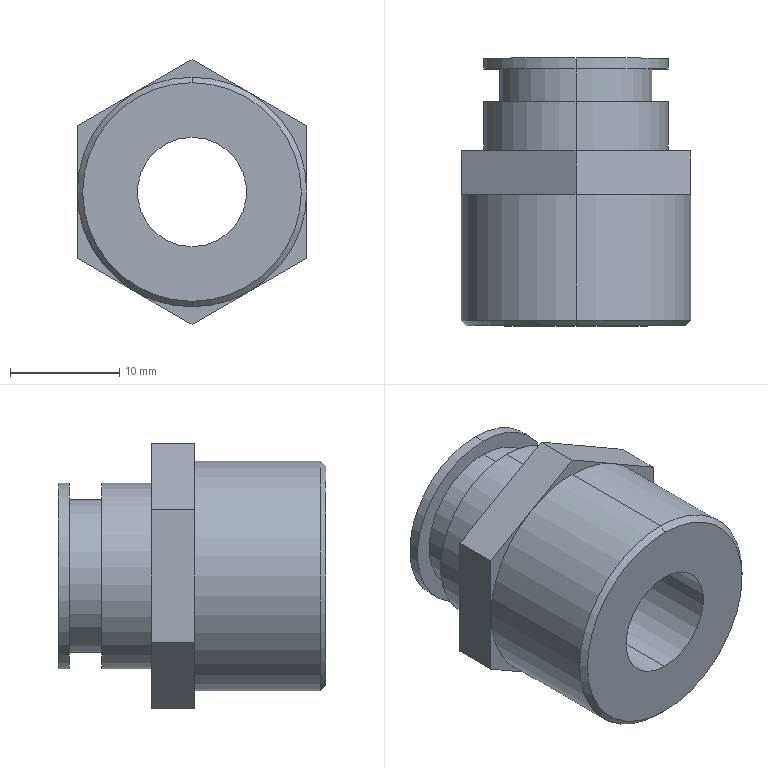Part | SolidWorks | features ICE 6, Chamfer 1, Extrusion 1 | 1 solid | 32 faces | box 21 x 24.5 x 24.249 mm | volume 5082 mm3 | plane 18 | cylinder 12 | cone 2 | commonest cylinder face diameters 17 x4 10 x2 12 x2 14 x2 21 x2
STEP:
#1=CARTESIAN_POINT('',(0.,13.5,-5.));
#2=VERTEX_POINT('',#1);
#3=CARTESIAN_POINT('',(0.,13.5,5.));
#4=VERTEX_POINT('',#3);
#5=CARTESIAN_POINT('',(0.,13.5,0.));
#6=DIRECTION('',(0.,1.,0.));
#7=DIRECTION('',(0.,0.,1.));
#8=AXIS2_PLACEMENT_3D('',#5,#6,#7);
#9=CIRCLE('',#8,5.);
#10=EDGE_CURVE('',#2,#4,#9,.T.);
#11=ORIENTED_EDGE('',*,*,#10,.T.);
#12=CARTESIAN_POINT('',(0.,0.,5.));
#13=VERTEX_POINT('',#12);
#14=CARTESIAN_POINT('',(0.,24.5,5.));
#15=DIRECTION('',(0.,-1.,0.));
#16=VECTOR('',#15,1000.);
#17=LINE('',#14,#16);
#18=EDGE_CURVE('',#4,#13,#17,.T.);
#19=ORIENTED_EDGE('',*,*,#18,.T.);
#20=CARTESIAN_POINT('',(0.,0.,-5.));
#21=VERTEX_POINT('',#20);
#22=CARTESIAN_POINT('',(0.,0.,0.));
#23=DIRECTION('',(0.,-1.,0.));
#24=DIRECTION('',(0.,0.,-1.));
#25=AXIS2_PLACEMENT_3D('',#22,#23,#24);
#26=CIRCLE('',#25,5.);
#27=EDGE_CURVE('',#13,#21,#26,.T.);
#28=ORIENTED_EDGE('',*,*,#27,.T.);
#29=CARTESIAN_POINT('',(0.,24.5,-5.));
#30=DIRECTION('',(0.,-1.,0.));
#31=VECTOR('',#30,1000.);
#32=LINE('',#29,#31);
#33=EDGE_CURVE('',#2,#21,#32,.T.);
#34=ORIENTED_EDGE('',*,*,#33,.F.);
#35=EDGE_LOOP('',(#11,#19,#28,#34));
#36=FACE_OUTER_BOUND('',#35,.T.);
#37=CARTESIAN_POINT('',(0.,24.5,0.));
#38=DIRECTION('',(0.,-1.,0.));
#39=DIRECTION('',(0.,0.,-1.));
#40=AXIS2_PLACEMENT_3D('',#37,#38,#39);
#41=CYLINDRICAL_SURFACE('',#40,5.);
#42=ADVANCED_FACE('',(#36),#41,.F.);
#43=CARTESIAN_POINT('',(0.,13.5,-6.));
#44=VERTEX_POINT('',#43);
#45=CARTESIAN_POINT('',(0.,13.5,6.));
#46=VERTEX_POINT('',#45);
#47=CARTESIAN_POINT('',(0.,13.5,0.));
#48=DIRECTION('',(0.,1.,0.));
#49=DIRECTION('',(0.,0.,1.));
#50=AXIS2_PLACEMENT_3D('',#47,#48,#49);
#51=CIRCLE('',#50,6.);
#52=EDGE_CURVE('',#44,#46,#51,.T.);
#53=ORIENTED_EDGE('',*,*,#52,.F.);
#54=CARTESIAN_POINT('',(0.,24.5,-6.));
#55=VERTEX_POINT('',#54);
#56=CARTESIAN_POINT('',(0.,13.5,-6.));
#57=DIRECTION('',(0.,1.,0.));
#58=VECTOR('',#57,1000.);
#59=LINE('',#56,#58);
#60=EDGE_CURVE('',#44,#55,#59,.T.);
#61=ORIENTED_EDGE('',*,*,#60,.T.);
#62=CARTESIAN_POINT('',(0.,24.5,6.));
#63=VERTEX_POINT('',#62);
#64=CARTESIAN_POINT('',(0.,24.5,0.));
#65=DIRECTION('',(0.,1.,0.));
#66=DIRECTION('',(0.,0.,1.));
#67=AXIS2_PLACEMENT_3D('',#64,#65,#66);
#68=CIRCLE('',#67,6.);
#69=EDGE_CURVE('',#55,#63,#68,.T.);
#70=ORIENTED_EDGE('',*,*,#69,.T.);
#71=CARTESIAN_POINT('',(0.,13.5,6.));
#72=DIRECTION('',(0.,1.,0.));
#73=VECTOR('',#72,1000.);
#74=LINE('',#71,#73);
#75=EDGE_CURVE('',#46,#63,#74,.T.);
#76=ORIENTED_EDGE('',*,*,#75,.F.);
#77=EDGE_LOOP('',(#53,#61,#70,#76));
#78=FACE_OUTER_BOUND('',#77,.T.);
#79=CARTESIAN_POINT('',(0.,13.5,0.));
#80=DIRECTION('',(0.,1.,0.));
#81=DIRECTION('',(0.,0.,1.));
#82=AXIS2_PLACEMENT_3D('',#79,#80,#81);
#83=CYLINDRICAL_SURFACE('',#82,6.);
#84=ADVANCED_FACE('',(#78),#83,.F.);
#85=CARTESIAN_POINT('',(0.,0.,-10.));
#86=VERTEX_POINT('',#85);
#87=CARTESIAN_POINT('',(0.,0.,10.));
#88=VERTEX_POINT('',#87);
#89=CARTESIAN_POINT('',(0.,0.,0.));
#90=DIRECTION('',(0.,-1.,0.));
#91=DIRECTION('',(0.,0.,1.));
#92=AXIS2_PLACEMENT_3D('',#89,#90,#91);
#93=CIRCLE('',#92,10.);
#94=EDGE_CURVE('',#86,#88,#93,.T.);
#95=ORIENTED_EDGE('',*,*,#94,.F.);
#96=CARTESIAN_POINT('',(0.,0.5,-10.5));
#97=VERTEX_POINT('',#96);
#98=CARTESIAN_POINT('',(0.,0.5,-10.5));
#99=DIRECTION('',(0.,0.7071,-0.7071));
#100=VECTOR('',#99,1000.);
#101=LINE('',#98,#100);
#102=EDGE_CURVE('',#86,#97,#101,.T.);
#103=ORIENTED_EDGE('',*,*,#102,.T.);
#104=CARTESIAN_POINT('',(0.,0.5,10.5));
#105=VERTEX_POINT('',#104);
#106=CARTESIAN_POINT('',(0.,0.5,0.));
#107=DIRECTION('',(0.,1.,0.));
#108=DIRECTION('',(0.,0.,1.));
#109=AXIS2_PLACEMENT_3D('',#106,#107,#108);
#110=CIRCLE('',#109,10.5);
#111=EDGE_CURVE('',#105,#97,#110,.T.);
#112=ORIENTED_EDGE('',*,*,#111,.F.);
#113=CARTESIAN_POINT('',(0.,0.5,10.5));
#114=DIRECTION('',(0.,0.7071,0.7071));
#115=VECTOR('',#114,1000.);
#116=LINE('',#113,#115);
#117=EDGE_CURVE('',#88,#105,#116,.T.);
#118=ORIENTED_EDGE('',*,*,#117,.F.);
#119=EDGE_LOOP('',(#95,#103,#112,#118));
#120=FACE_OUTER_BOUND('',#119,.T.);
#121=CARTESIAN_POINT('',(0.,0.5,0.));
#122=DIRECTION('',(0.,1.,0.));
#123=DIRECTION('',(0.,0.,1.));
#124=AXIS2_PLACEMENT_3D('',#121,#122,#123);
#125=CONICAL_SURFACE('',#124,10.5,0.7854);
#126=ADVANCED_FACE('',(#120),#125,.T.);
#127=CARTESIAN_POINT('',(0.,24.5,8.5));
#128=VERTEX_POINT('',#127);
#129=CARTESIAN_POINT('',(0.,24.5,-8.5));
#130=VERTEX_POINT('',#129);
#131=CARTESIAN_POINT('',(0.,24.5,0.));
#132=DIRECTION('',(0.,1.,0.));
#133=DIRECTION('',(0.,0.,1.));
#134=AXIS2_PLACEMENT_3D('',#131,#132,#133);
#135=CIRCLE('',#134,8.5);
#136=EDGE_CURVE('',#128,#130,#135,.T.);
#137=ORIENTED_EDGE('',*,*,#136,.F.);
#138=CARTESIAN_POINT('',(0.,23.5,8.5));
#139=VERTEX_POINT('',#138);
#140=CARTESIAN_POINT('',(0.,24.5,8.5));
#141=DIRECTION('',(0.,-1.,0.));
#142=VECTOR('',#141,1000.);
#143=LINE('',#140,#142);
#144=EDGE_CURVE('',#128,#139,#143,.T.);
#145=ORIENTED_EDGE('',*,*,#144,.T.);
#146=CARTESIAN_POINT('',(0.,23.5,-8.5));
#147=VERTEX_POINT('',#146);
#148=CARTESIAN_POINT('',(0.,23.5,0.));
#149=DIRECTION('',(0.,1.,0.));
#150=DIRECTION('',(0.,0.,1.));
#151=AXIS2_PLACEMENT_3D('',#148,#149,#150);
#152=CIRCLE('',#151,8.5);
#153=EDGE_CURVE('',#139,#147,#152,.T.);
#154=ORIENTED_EDGE('',*,*,#153,.T.);
#155=CARTESIAN_POINT('',(0.,24.5,-8.5));
#156=DIRECTION('',(0.,-1.,0.));
#157=VECTOR('',#156,1000.);
#158=LINE('',#155,#157);
#159=EDGE_CURVE('',#130,#147,#158,.T.);
#160=ORIENTED_EDGE('',*,*,#159,.F.);
#161=EDGE_LOOP('',(#137,#145,#154,#160));
#162=FACE_OUTER_BOUND('',#161,.T.);
#163=CARTESIAN_POINT('',(0.,24.5,0.));
#164=DIRECTION('',(0.,-1.,0.));
#165=DIRECTION('',(0.,0.,-1.));
#166=AXIS2_PLACEMENT_3D('',#163,#164,#165);
#167=CYLINDRICAL_SURFACE('',#166,8.5);
#168=ADVANCED_FACE('',(#162),#167,.T.);
#169=CARTESIAN_POINT('',(0.,23.5,7.));
#170=VERTEX_POINT('',#169);
#171=CARTESIAN_POINT('',(0.,23.5,-7.));
#172=VERTEX_POINT('',#171);
#173=CARTESIAN_POINT('',(0.,23.5,0.));
#174=DIRECTION('',(0.,1.,0.));
#175=DIRECTION('',(0.,0.,1.));
#176=AXIS2_PLACEMENT_3D('',#173,#174,#175);
#177=CIRCLE('',#176,7.);
#178=EDGE_CURVE('',#170,#172,#177,.T.);
#179=ORIENTED_EDGE('',*,*,#178,.F.);
#180=CARTESIAN_POINT('',(0.,20.5,7.));
#181=VERTEX_POINT('',#180);
#182=CARTESIAN_POINT('',(0.,23.5,7.));
#183=DIRECTION('',(0.,-1.,0.));
#184=VECTOR('',#183,1000.);
#185=LINE('',#182,#184);
#186=EDGE_CURVE('',#170,#181,#185,.T.);
#187=ORIENTED_EDGE('',*,*,#186,.T.);
#188=CARTESIAN_POINT('',(0.,20.5,-7.));
#189=VERTEX_POINT('',#188);
#190=CARTESIAN_POINT('',(0.,20.5,0.));
#191=DIRECTION('',(0.,1.,0.));
#192=DIRECTION('',(0.,0.,1.));
#193=AXIS2_PLACEMENT_3D('',#190,#191,#192);
#194=CIRCLE('',#193,7.);
#195=EDGE_CURVE('',#181,#189,#194,.T.);
#196=ORIENTED_EDGE('',*,*,#195,.T.);
#197=CARTESIAN_POINT('',(0.,23.5,-7.));
#198=DIRECTION('',(0.,-1.,0.));
#199=VECTOR('',#198,1000.);
#200=LINE('',#197,#199);
#201=EDGE_CURVE('',#172,#189,#200,.T.);
#202=ORIENTED_EDGE('',*,*,#201,.F.);
#203=EDGE_LOOP('',(#179,#187,#196,#202));
#204=FACE_OUTER_BOUND('',#203,.T.);
#205=CARTESIAN_POINT('',(0.,23.5,0.));
#206=DIRECTION('',(0.,-1.,0.));
#207=DIRECTION('',(0.,0.,-1.));
#208=AXIS2_PLACEMENT_3D('',#205,#206,#207);
#209=CYLINDRICAL_SURFACE('',#208,7.);
#210=ADVANCED_FACE('',(#204),#209,.T.);
#211=CARTESIAN_POINT('',(0.,20.5,8.5));
#212=VERTEX_POINT('',#211);
#213=CARTESIAN_POINT('',(0.,20.5,-8.5));
#214=VERTEX_POINT('',#213);
#215=CARTESIAN_POINT('',(0.,20.5,0.));
#216=DIRECTION('',(0.,1.,0.));
#217=DIRECTION('',(0.,0.,1.));
#218=AXIS2_PLACEMENT_3D('',#215,#216,#217);
#219=CIRCLE('',#218,8.5);
#220=EDGE_CURVE('',#212,#214,#219,.T.);
#221=ORIENTED_EDGE('',*,*,#220,.F.);
#222=CARTESIAN_POINT('',(0.,16.,8.5));
#223=VERTEX_POINT('',#222);
#224=CARTESIAN_POINT('',(0.,20.5,8.5));
#225=DIRECTION('',(0.,-1.,0.));
#226=VECTOR('',#225,1000.);
#227=LINE('',#224,#226);
#228=EDGE_CURVE('',#212,#223,#227,.T.);
#229=ORIENTED_EDGE('',*,*,#228,.T.);
#230=CARTESIAN_POINT('',(0.,16.,-8.5));
#231=VERTEX_POINT('',#230);
#232=CARTESIAN_POINT('',(0.,16.,0.));
#233=DIRECTION('',(0.,1.,0.));
#234=DIRECTION('',(0.,0.,1.));
#235=AXIS2_PLACEMENT_3D('',#232,#233,#234);
#236=CIRCLE('',#235,8.5);
#237=EDGE_CURVE('',#223,#231,#236,.T.);
#238=ORIENTED_EDGE('',*,*,#237,.T.);
#239=CARTESIAN_POINT('',(0.,20.5,-8.5));
#240=DIRECTION('',(0.,-1.,0.));
#241=VECTOR('',#240,1000.);
#242=LINE('',#239,#241);
#243=EDGE_CURVE('',#214,#231,#242,.T.);
#244=ORIENTED_EDGE('',*,*,#243,.F.);
#245=EDGE_LOOP('',(#221,#229,#238,#244));
#246=FACE_OUTER_BOUND('',#245,.T.);
#247=CARTESIAN_POINT('',(0.,20.5,0.));
#248=DIRECTION('',(0.,-1.,0.));
#249=DIRECTION('',(0.,0.,-1.));
#250=AXIS2_PLACEMENT_3D('',#247,#248,#249);
#251=CYLINDRICAL_SURFACE('',#250,8.5);
#252=ADVANCED_FACE('',(#246),#251,.T.);
#253=CARTESIAN_POINT('',(0.,12.,10.5));
#254=VERTEX_POINT('',#253);
#255=CARTESIAN_POINT('',(5.25,12.,9.093));
#256=VERTEX_POINT('',#255);
#257=CARTESIAN_POINT('',(0.,12.,0.));
#258=DIRECTION('',(0.,1.,0.));
#259=DIRECTION('',(0.,0.,1.));
#260=AXIS2_PLACEMENT_3D('',#257,#258,#259);
#261=CIRCLE('',#260,10.5);
#262=EDGE_CURVE('',#254,#256,#261,.T.);
#263=ORIENTED_EDGE('',*,*,#262,.F.);
#264=CARTESIAN_POINT('',(0.,12.,10.5));
#265=DIRECTION('',(0.,-1.,0.));
#266=VECTOR('',#265,1000.);
#267=LINE('',#264,#266);
#268=EDGE_CURVE('',#254,#105,#267,.T.);
#269=ORIENTED_EDGE('',*,*,#268,.T.);
#270=ORIENTED_EDGE('',*,*,#111,.T.);
#271=CARTESIAN_POINT('',(0.,12.,-10.5));
#272=VERTEX_POINT('',#271);
#273=CARTESIAN_POINT('',(0.,12.,-10.5));
#274=DIRECTION('',(0.,-1.,0.));
#275=VECTOR('',#274,1000.);
#276=LINE('',#273,#275);
#277=EDGE_CURVE('',#272,#97,#276,.T.);
#278=ORIENTED_EDGE('',*,*,#277,.F.);
#279=CARTESIAN_POINT('',(5.25,12.,-9.093));
#280=VERTEX_POINT('',#279);
#281=CARTESIAN_POINT('',(0.,12.,0.));
#282=DIRECTION('',(0.,1.,0.));
#283=DIRECTION('',(0.,0.,1.));
#284=AXIS2_PLACEMENT_3D('',#281,#282,#283);
#285=CIRCLE('',#284,10.5);
#286=EDGE_CURVE('',#280,#272,#285,.T.);
#287=ORIENTED_EDGE('',*,*,#286,.F.);
#288=CARTESIAN_POINT('',(10.5,12.,0.));
#289=VERTEX_POINT('',#288);
#290=CARTESIAN_POINT('',(0.,12.,0.));
#291=DIRECTION('',(0.,1.,0.));
#292=DIRECTION('',(0.,0.,1.));
#293=AXIS2_PLACEMENT_3D('',#290,#291,#292);
#294=CIRCLE('',#293,10.5);
#295=EDGE_CURVE('',#289,#280,#294,.T.);
#296=ORIENTED_EDGE('',*,*,#295,.F.);
#297=CARTESIAN_POINT('',(0.,12.,0.));
#298=DIRECTION('',(0.,1.,0.));
#299=DIRECTION('',(0.,0.,1.));
#300=AXIS2_PLACEMENT_3D('',#297,#298,#299);
#301=CIRCLE('',#300,10.5);
#302=EDGE_CURVE('',#256,#289,#301,.T.);
#303=ORIENTED_EDGE('',*,*,#302,.F.);
#304=EDGE_LOOP('',(#263,#269,#270,#278,#287,#296,#303));
#305=FACE_OUTER_BOUND('',#304,.T.);
#306=CARTESIAN_POINT('',(0.,12.,0.));
#307=DIRECTION('',(0.,-1.,0.));
#308=DIRECTION('',(0.,0.,-1.));
#309=AXIS2_PLACEMENT_3D('',#306,#307,#308);
#310=CYLINDRICAL_SURFACE('',#309,10.5);
#311=ADVANCED_FACE('',(#305),#310,.T.);
#312=ORIENTED_EDGE('',*,*,#268,.F.);
#313=CARTESIAN_POINT('',(-5.25,12.,9.093));
#314=VERTEX_POINT('',#313);
#315=CARTESIAN_POINT('',(0.,12.,0.));
#316=DIRECTION('',(0.,1.,0.));
#317=DIRECTION('',(0.,0.,1.));
#318=AXIS2_PLACEMENT_3D('',#315,#316,#317);
#319=CIRCLE('',#318,10.5);
#320=EDGE_CURVE('',#314,#254,#319,.T.);
#321=ORIENTED_EDGE('',*,*,#320,.F.);
#322=CARTESIAN_POINT('',(-10.5,12.,0.));
#323=VERTEX_POINT('',#322);
#324=CARTESIAN_POINT('',(0.,12.,0.));
#325=DIRECTION('',(0.,1.,0.));
#326=DIRECTION('',(0.,0.,1.));
#327=AXIS2_PLACEMENT_3D('',#324,#325,#326);
#328=CIRCLE('',#327,10.5);
#329=EDGE_CURVE('',#323,#314,#328,.T.);
#330=ORIENTED_EDGE('',*,*,#329,.F.);
#331=CARTESIAN_POINT('',(-5.25,12.,-9.093));
#332=VERTEX_POINT('',#331);
#333=CARTESIAN_POINT('',(0.,12.,0.));
#334=DIRECTION('',(0.,1.,0.));
#335=DIRECTION('',(0.,0.,1.));
#336=AXIS2_PLACEMENT_3D('',#333,#334,#335);
#337=CIRCLE('',#336,10.5);
#338=EDGE_CURVE('',#332,#323,#337,.T.);
#339=ORIENTED_EDGE('',*,*,#338,.F.);
#340=CARTESIAN_POINT('',(0.,12.,0.));
#341=DIRECTION('',(0.,1.,0.));
#342=DIRECTION('',(0.,0.,1.));
#343=AXIS2_PLACEMENT_3D('',#340,#341,#342);
#344=CIRCLE('',#343,10.5);
#345=EDGE_CURVE('',#272,#332,#344,.T.);
#346=ORIENTED_EDGE('',*,*,#345,.F.);
#347=ORIENTED_EDGE('',*,*,#277,.T.);
#348=CARTESIAN_POINT('',(0.,0.5,0.));
#349=DIRECTION('',(0.,1.,0.));
#350=DIRECTION('',(0.,0.,1.));
#351=AXIS2_PLACEMENT_3D('',#348,#349,#350);
#352=CIRCLE('',#351,10.5);
#353=EDGE_CURVE('',#97,#105,#352,.T.);
#354=ORIENTED_EDGE('',*,*,#353,.T.);
#355=EDGE_LOOP('',(#312,#321,#330,#339,#346,#347,#354));
#356=FACE_OUTER_BOUND('',#355,.T.);
#357=CARTESIAN_POINT('',(0.,12.,0.));
#358=DIRECTION('',(0.,-1.,0.));
#359=DIRECTION('',(0.,0.,-1.));
#360=AXIS2_PLACEMENT_3D('',#357,#358,#359);
#361=CYLINDRICAL_SURFACE('',#360,10.5);
#362=ADVANCED_FACE('',(#356),#361,.T.);
#363=CARTESIAN_POINT('',(0.,0.,0.));
#364=DIRECTION('',(0.,-1.,0.));
#365=DIRECTION('',(0.,0.,-1.));
#366=AXIS2_PLACEMENT_3D('',#363,#364,#365);
#367=CIRCLE('',#366,5.);
#368=EDGE_CURVE('',#21,#13,#367,.T.);
#369=ORIENTED_EDGE('',*,*,#368,.F.);
#370=ORIENTED_EDGE('',*,*,#27,.F.);
#371=EDGE_LOOP('',(#369,#370));
#372=FACE_BOUND('',#371,.T.);
#373=CARTESIAN_POINT('',(0.,0.,0.));
#374=DIRECTION('',(0.,-1.,0.));
#375=DIRECTION('',(0.,0.,1.));
#376=AXIS2_PLACEMENT_3D('',#373,#374,#375);
#377=CIRCLE('',#376,10.);
#378=EDGE_CURVE('',#88,#86,#377,.T.);
#379=ORIENTED_EDGE('',*,*,#378,.T.);
#380=ORIENTED_EDGE('',*,*,#94,.T.);
#381=EDGE_LOOP('',(#379,#380));
#382=FACE_OUTER_BOUND('',#381,.T.);
#383=CARTESIAN_POINT('',(0.,0.,0.));
#384=DIRECTION('',(0.,1.,0.));
#385=DIRECTION('',(0.,0.,1.));
#386=AXIS2_PLACEMENT_3D('',#383,#384,#385);
#387=PLANE('',#386);
#388=ADVANCED_FACE('',(#372,#382),#387,.F.);
#389=CARTESIAN_POINT('',(10.5,12.,6.062));
#390=VERTEX_POINT('',#389);
#391=CARTESIAN_POINT('',(0.,12.,12.124));
#392=DIRECTION('',(0.866,0.,-0.5));
#393=VECTOR('',#392,1000.);
#394=LINE('',#391,#393);
#395=EDGE_CURVE('',#256,#390,#394,.T.);
#396=ORIENTED_EDGE('',*,*,#395,.F.);
#397=ORIENTED_EDGE('',*,*,#302,.T.);
#398=CARTESIAN_POINT('',(10.5,12.,6.062));
#399=DIRECTION('',(0.,0.,-1.));
#400=VECTOR('',#399,1000.);
#401=LINE('',#398,#400);
#402=EDGE_CURVE('',#390,#289,#401,.T.);
#403=ORIENTED_EDGE('',*,*,#402,.F.);
#404=EDGE_LOOP('',(#396,#397,#403));
#405=FACE_OUTER_BOUND('',#404,.T.);
#406=CARTESIAN_POINT('',(0.,12.,0.));
#407=DIRECTION('',(0.,1.,0.));
#408=DIRECTION('',(0.,0.,1.));
#409=AXIS2_PLACEMENT_3D('',#406,#407,#408);
#410=PLANE('',#409);
#411=ADVANCED_FACE('',(#405),#410,.F.);
#412=CARTESIAN_POINT('',(10.5,12.,-6.062));
#413=VERTEX_POINT('',#412);
#414=CARTESIAN_POINT('',(10.5,12.,6.062));
#415=DIRECTION('',(0.,0.,-1.));
#416=VECTOR('',#415,1000.);
#417=LINE('',#414,#416);
#418=EDGE_CURVE('',#289,#413,#417,.T.);
#419=ORIENTED_EDGE('',*,*,#418,.F.);
#420=ORIENTED_EDGE('',*,*,#295,.T.);
#421=CARTESIAN_POINT('',(10.5,12.,-6.062));
#422=DIRECTION('',(-0.866,0.,-0.5));
#423=VECTOR('',#422,1000.);
#424=LINE('',#421,#423);
#425=EDGE_CURVE('',#413,#280,#424,.T.);
#426=ORIENTED_EDGE('',*,*,#425,.F.);
#427=EDGE_LOOP('',(#419,#420,#426));
#428=FACE_OUTER_BOUND('',#427,.T.);
#429=CARTESIAN_POINT('',(0.,12.,0.));
#430=DIRECTION('',(0.,1.,0.));
#431=DIRECTION('',(0.,0.,1.));
#432=AXIS2_PLACEMENT_3D('',#429,#430,#431);
#433=PLANE('',#432);
#434=ADVANCED_FACE('',(#428),#433,.F.);
#435=CARTESIAN_POINT('',(0.,12.,-12.124));
#436=VERTEX_POINT('',#435);
#437=CARTESIAN_POINT('',(10.5,12.,-6.062));
#438=DIRECTION('',(-0.866,0.,-0.5));
#439=VECTOR('',#438,1000.);
#440=LINE('',#437,#439);
#441=EDGE_CURVE('',#280,#436,#440,.T.);
#442=ORIENTED_EDGE('',*,*,#441,.F.);
#443=ORIENTED_EDGE('',*,*,#286,.T.);
#444=ORIENTED_EDGE('',*,*,#345,.T.);
#445=CARTESIAN_POINT('',(0.,12.,-12.124));
#446=DIRECTION('',(-0.866,0.,0.5));
#447=VECTOR('',#446,1000.);
#448=LINE('',#445,#447);
#449=EDGE_CURVE('',#436,#332,#448,.T.);
#450=ORIENTED_EDGE('',*,*,#449,.F.);
#451=EDGE_LOOP('',(#442,#443,#444,#450));
#452=FACE_OUTER_BOUND('',#451,.T.);
#453=CARTESIAN_POINT('',(0.,12.,0.));
#454=DIRECTION('',(0.,1.,0.));
#455=DIRECTION('',(0.,0.,1.));
#456=AXIS2_PLACEMENT_3D('',#453,#454,#455);
#457=PLANE('',#456);
#458=ADVANCED_FACE('',(#452),#457,.F.);
#459=CARTESIAN_POINT('',(-10.5,12.,-6.062));
#460=VERTEX_POINT('',#459);
#461=CARTESIAN_POINT('',(0.,12.,-12.124));
#462=DIRECTION('',(-0.866,0.,0.5));
#463=VECTOR('',#462,1000.);
#464=LINE('',#461,#463);
#465=EDGE_CURVE('',#332,#460,#464,.T.);
#466=ORIENTED_EDGE('',*,*,#465,.F.);
#467=ORIENTED_EDGE('',*,*,#338,.T.);
#468=CARTESIAN_POINT('',(-10.5,12.,-6.062));
#469=DIRECTION('',(0.,0.,1.));
#470=VECTOR('',#469,1000.);
#471=LINE('',#468,#470);
#472=EDGE_CURVE('',#460,#323,#471,.T.);
#473=ORIENTED_EDGE('',*,*,#472,.F.);
#474=EDGE_LOOP('',(#466,#467,#473));
#475=FACE_OUTER_BOUND('',#474,.T.);
#476=CARTESIAN_POINT('',(0.,12.,0.));
#477=DIRECTION('',(0.,1.,0.));
#478=DIRECTION('',(0.,0.,1.));
#479=AXIS2_PLACEMENT_3D('',#476,#477,#478);
#480=PLANE('',#479);
#481=ADVANCED_FACE('',(#475),#480,.F.);
#482=CARTESIAN_POINT('',(-10.5,12.,6.062));
#483=VERTEX_POINT('',#482);
#484=CARTESIAN_POINT('',(-10.5,12.,-6.062));
#485=DIRECTION('',(0.,0.,1.));
#486=VECTOR('',#485,1000.);
#487=LINE('',#484,#486);
#488=EDGE_CURVE('',#323,#483,#487,.T.);
#489=ORIENTED_EDGE('',*,*,#488,.F.);
#490=ORIENTED_EDGE('',*,*,#329,.T.);
#491=CARTESIAN_POINT('',(-10.5,12.,6.062));
#492=DIRECTION('',(0.866,0.,0.5));
#493=VECTOR('',#492,1000.);
#494=LINE('',#491,#493);
#495=EDGE_CURVE('',#483,#314,#494,.T.);
#496=ORIENTED_EDGE('',*,*,#495,.F.);
#497=EDGE_LOOP('',(#489,#490,#496));
#498=FACE_OUTER_BOUND('',#497,.T.);
#499=CARTESIAN_POINT('',(0.,12.,0.));
#500=DIRECTION('',(0.,1.,0.));
#501=DIRECTION('',(0.,0.,1.));
#502=AXIS2_PLACEMENT_3D('',#499,#500,#501);
#503=PLANE('',#502);
#504=ADVANCED_FACE('',(#498),#503,.F.);
#505=CARTESIAN_POINT('',(0.,12.,12.124));
#506=VERTEX_POINT('',#505);
#507=CARTESIAN_POINT('',(-10.5,12.,6.062));
#508=DIRECTION('',(0.866,0.,0.5));
#509=VECTOR('',#508,1000.);
#510=LINE('',#507,#509);
#511=EDGE_CURVE('',#314,#506,#510,.T.);
#512=ORIENTED_EDGE('',*,*,#511,.F.);
#513=ORIENTED_EDGE('',*,*,#320,.T.);
#514=ORIENTED_EDGE('',*,*,#262,.T.);
#515=CARTESIAN_POINT('',(0.,12.,12.124));
#516=DIRECTION('',(0.866,0.,-0.5));
#517=VECTOR('',#516,1000.);
#518=LINE('',#515,#517);
#519=EDGE_CURVE('',#506,#256,#518,.T.);
#520=ORIENTED_EDGE('',*,*,#519,.F.);
#521=EDGE_LOOP('',(#512,#513,#514,#520));
#522=FACE_OUTER_BOUND('',#521,.T.);
#523=CARTESIAN_POINT('',(0.,12.,0.));
#524=DIRECTION('',(0.,1.,0.));
#525=DIRECTION('',(0.,0.,1.));
#526=AXIS2_PLACEMENT_3D('',#523,#524,#525);
#527=PLANE('',#526);
#528=ADVANCED_FACE('',(#522),#527,.F.);
#529=ORIENTED_EDGE('',*,*,#519,.T.);
#530=ORIENTED_EDGE('',*,*,#395,.T.);
#531=CARTESIAN_POINT('',(10.5,16.,6.062));
#532=VERTEX_POINT('',#531);
#533=CARTESIAN_POINT('',(10.5,16.,6.062));
#534=DIRECTION('',(0.,-1.,0.));
#535=VECTOR('',#534,1000.);
#536=LINE('',#533,#535);
#537=EDGE_CURVE('',#532,#390,#536,.T.);
#538=ORIENTED_EDGE('',*,*,#537,.F.);
#539=CARTESIAN_POINT('',(0.,16.,12.124));
#540=VERTEX_POINT('',#539);
#541=CARTESIAN_POINT('',(0.,16.,12.124));
#542=DIRECTION('',(0.866,0.,-0.5));
#543=VECTOR('',#542,1000.);
#544=LINE('',#541,#543);
#545=EDGE_CURVE('',#540,#532,#544,.T.);
#546=ORIENTED_EDGE('',*,*,#545,.F.);
#547=CARTESIAN_POINT('',(0.,16.,12.124));
#548=DIRECTION('',(0.,-1.,0.));
#549=VECTOR('',#548,1000.);
#550=LINE('',#547,#549);
#551=EDGE_CURVE('',#540,#506,#550,.T.);
#552=ORIENTED_EDGE('',*,*,#551,.T.);
#553=EDGE_LOOP('',(#529,#530,#538,#546,#552));
#554=FACE_OUTER_BOUND('',#553,.T.);
#555=CARTESIAN_POINT('',(0.,16.,12.124));
#556=DIRECTION('',(-0.5,0.,-0.866));
#557=DIRECTION('',(-0.866,0.,0.5));
#558=AXIS2_PLACEMENT_3D('',#555,#556,#557);
#559=PLANE('',#558);
#560=ADVANCED_FACE('',(#554),#559,.F.);
#561=ORIENTED_EDGE('',*,*,#402,.T.);
#562=ORIENTED_EDGE('',*,*,#418,.T.);
#563=CARTESIAN_POINT('',(10.5,16.,-6.062));
#564=VERTEX_POINT('',#563);
#565=CARTESIAN_POINT('',(10.5,16.,-6.062));
#566=DIRECTION('',(0.,-1.,0.));
#567=VECTOR('',#566,1000.);
#568=LINE('',#565,#567);
#569=EDGE_CURVE('',#564,#413,#568,.T.);
#570=ORIENTED_EDGE('',*,*,#569,.F.);
#571=CARTESIAN_POINT('',(10.5,16.,6.062));
#572=DIRECTION('',(0.,0.,-1.));
#573=VECTOR('',#572,1000.);
#574=LINE('',#571,#573);
#575=EDGE_CURVE('',#532,#564,#574,.T.);
#576=ORIENTED_EDGE('',*,*,#575,.F.);
#577=ORIENTED_EDGE('',*,*,#537,.T.);
#578=EDGE_LOOP('',(#561,#562,#570,#576,#577));
#579=FACE_OUTER_BOUND('',#578,.T.);
#580=CARTESIAN_POINT('',(10.5,16.,6.062));
#581=DIRECTION('',(-1.,0.,0.));
#582=DIRECTION('',(0.,0.,1.));
#583=AXIS2_PLACEMENT_3D('',#580,#581,#582);
#584=PLANE('',#583);
#585=ADVANCED_FACE('',(#579),#584,.F.);
#586=ORIENTED_EDGE('',*,*,#425,.T.);
#587=ORIENTED_EDGE('',*,*,#441,.T.);
#588=CARTESIAN_POINT('',(0.,16.,-12.124));
#589=VERTEX_POINT('',#588);
#590=CARTESIAN_POINT('',(0.,16.,-12.124));
#591=DIRECTION('',(0.,-1.,0.));
#592=VECTOR('',#591,1000.);
#593=LINE('',#590,#592);
#594=EDGE_CURVE('',#589,#436,#593,.T.);
#595=ORIENTED_EDGE('',*,*,#594,.F.);
#596=CARTESIAN_POINT('',(10.5,16.,-6.062));
#597=DIRECTION('',(-0.866,0.,-0.5));
#598=VECTOR('',#597,1000.);
#599=LINE('',#596,#598);
#600=EDGE_CURVE('',#564,#589,#599,.T.);
#601=ORIENTED_EDGE('',*,*,#600,.F.);
#602=ORIENTED_EDGE('',*,*,#569,.T.);
#603=EDGE_LOOP('',(#586,#587,#595,#601,#602));
#604=FACE_OUTER_BOUND('',#603,.T.);
#605=CARTESIAN_POINT('',(10.5,16.,-6.062));
#606=DIRECTION('',(-0.5,0.,0.866));
#607=DIRECTION('',(0.866,0.,0.5));
#608=AXIS2_PLACEMENT_3D('',#605,#606,#607);
#609=PLANE('',#608);
#610=ADVANCED_FACE('',(#604),#609,.F.);
#611=ORIENTED_EDGE('',*,*,#449,.T.);
#612=ORIENTED_EDGE('',*,*,#465,.T.);
#613=CARTESIAN_POINT('',(-10.5,16.,-6.062));
#614=VERTEX_POINT('',#613);
#615=CARTESIAN_POINT('',(-10.5,16.,-6.062));
#616=DIRECTION('',(0.,-1.,0.));
#617=VECTOR('',#616,1000.);
#618=LINE('',#615,#617);
#619=EDGE_CURVE('',#614,#460,#618,.T.);
#620=ORIENTED_EDGE('',*,*,#619,.F.);
#621=CARTESIAN_POINT('',(0.,16.,-12.124));
#622=DIRECTION('',(-0.866,0.,0.5));
#623=VECTOR('',#622,1000.);
#624=LINE('',#621,#623);
#625=EDGE_CURVE('',#589,#614,#624,.T.);
#626=ORIENTED_EDGE('',*,*,#625,.F.);
#627=ORIENTED_EDGE('',*,*,#594,.T.);
#628=EDGE_LOOP('',(#611,#612,#620,#626,#627));
#629=FACE_OUTER_BOUND('',#628,.T.);
#630=CARTESIAN_POINT('',(0.,16.,-12.124));
#631=DIRECTION('',(0.5,0.,0.866));
#632=DIRECTION('',(0.866,0.,-0.5));
#633=AXIS2_PLACEMENT_3D('',#630,#631,#632);
#634=PLANE('',#633);
#635=ADVANCED_FACE('',(#629),#634,.F.);
#636=ORIENTED_EDGE('',*,*,#472,.T.);
#637=ORIENTED_EDGE('',*,*,#488,.T.);
#638=CARTESIAN_POINT('',(-10.5,16.,6.062));
#639=VERTEX_POINT('',#638);
#640=CARTESIAN_POINT('',(-10.5,16.,6.062));
#641=DIRECTION('',(0.,-1.,0.));
#642=VECTOR('',#641,1000.);
#643=LINE('',#640,#642);
#644=EDGE_CURVE('',#639,#483,#643,.T.);
#645=ORIENTED_EDGE('',*,*,#644,.F.);
#646=CARTESIAN_POINT('',(-10.5,16.,-6.062));
#647=DIRECTION('',(0.,0.,1.));
#648=VECTOR('',#647,1000.);
#649=LINE('',#646,#648);
#650=EDGE_CURVE('',#614,#639,#649,.T.);
#651=ORIENTED_EDGE('',*,*,#650,.F.);
#652=ORIENTED_EDGE('',*,*,#619,.T.);
#653=EDGE_LOOP('',(#636,#637,#645,#651,#652));
#654=FACE_OUTER_BOUND('',#653,.T.);
#655=CARTESIAN_POINT('',(-10.5,16.,-6.062));
#656=DIRECTION('',(1.,0.,0.));
#657=DIRECTION('',(0.,0.,-1.));
#658=AXIS2_PLACEMENT_3D('',#655,#656,#657);
#659=PLANE('',#658);
#660=ADVANCED_FACE('',(#654),#659,.F.);
#661=ORIENTED_EDGE('',*,*,#495,.T.);
#662=ORIENTED_EDGE('',*,*,#511,.T.);
#663=ORIENTED_EDGE('',*,*,#551,.F.);
#664=CARTESIAN_POINT('',(-10.5,16.,6.062));
#665=DIRECTION('',(0.866,0.,0.5));
#666=VECTOR('',#665,1000.);
#667=LINE('',#664,#666);
#668=EDGE_CURVE('',#639,#540,#667,.T.);
#669=ORIENTED_EDGE('',*,*,#668,.F.);
#670=ORIENTED_EDGE('',*,*,#644,.T.);
#671=EDGE_LOOP('',(#661,#662,#663,#669,#670));
#672=FACE_OUTER_BOUND('',#671,.T.);
#673=CARTESIAN_POINT('',(-10.5,16.,6.062));
#674=DIRECTION('',(0.5,0.,-0.866));
#675=DIRECTION('',(-0.866,0.,-0.5));
#676=AXIS2_PLACEMENT_3D('',#673,#674,#675);
#677=PLANE('',#676);
#678=ADVANCED_FACE('',(#672),#677,.F.);
#679=CARTESIAN_POINT('',(0.,16.,0.));
#680=DIRECTION('',(0.,1.,0.));
#681=DIRECTION('',(0.,0.,1.));
#682=AXIS2_PLACEMENT_3D('',#679,#680,#681);
#683=CIRCLE('',#682,8.5);
#684=EDGE_CURVE('',#231,#223,#683,.T.);
#685=ORIENTED_EDGE('',*,*,#684,.F.);
#686=ORIENTED_EDGE('',*,*,#237,.F.);
#687=EDGE_LOOP('',(#685,#686));
#688=FACE_BOUND('',#687,.T.);
#689=ORIENTED_EDGE('',*,*,#545,.T.);
#690=ORIENTED_EDGE('',*,*,#575,.T.);
#691=ORIENTED_EDGE('',*,*,#600,.T.);
#692=ORIENTED_EDGE('',*,*,#625,.T.);
#693=ORIENTED_EDGE('',*,*,#650,.T.);
#694=ORIENTED_EDGE('',*,*,#668,.T.);
#695=EDGE_LOOP('',(#689,#690,#691,#692,#693,#694));
#696=FACE_OUTER_BOUND('',#695,.T.);
#697=CARTESIAN_POINT('',(0.,16.,0.));
#698=DIRECTION('',(0.,1.,0.));
#699=DIRECTION('',(0.,0.,1.));
#700=AXIS2_PLACEMENT_3D('',#697,#698,#699);
#701=PLANE('',#700);
#702=ADVANCED_FACE('',(#688,#696),#701,.T.);
#703=ORIENTED_EDGE('',*,*,#228,.F.);
#704=CARTESIAN_POINT('',(0.,20.5,0.));
#705=DIRECTION('',(0.,1.,0.));
#706=DIRECTION('',(0.,0.,1.));
#707=AXIS2_PLACEMENT_3D('',#704,#705,#706);
#708=CIRCLE('',#707,8.5);
#709=EDGE_CURVE('',#214,#212,#708,.T.);
#710=ORIENTED_EDGE('',*,*,#709,.F.);
#711=ORIENTED_EDGE('',*,*,#243,.T.);
#712=ORIENTED_EDGE('',*,*,#684,.T.);
#713=EDGE_LOOP('',(#703,#710,#711,#712));
#714=FACE_OUTER_BOUND('',#713,.T.);
#715=CARTESIAN_POINT('',(0.,20.5,0.));
#716=DIRECTION('',(0.,-1.,0.));
#717=DIRECTION('',(0.,0.,-1.));
#718=AXIS2_PLACEMENT_3D('',#715,#716,#717);
#719=CYLINDRICAL_SURFACE('',#718,8.5);
#720=ADVANCED_FACE('',(#714),#719,.T.);
#721=CARTESIAN_POINT('',(0.,20.5,0.));
#722=DIRECTION('',(0.,1.,0.));
#723=DIRECTION('',(0.,0.,1.));
#724=AXIS2_PLACEMENT_3D('',#721,#722,#723);
#725=CIRCLE('',#724,7.);
#726=EDGE_CURVE('',#189,#181,#725,.T.);
#727=ORIENTED_EDGE('',*,*,#726,.F.);
#728=ORIENTED_EDGE('',*,*,#195,.F.);
#729=EDGE_LOOP('',(#727,#728));
#730=FACE_BOUND('',#729,.T.);
#731=ORIENTED_EDGE('',*,*,#709,.T.);
#732=ORIENTED_EDGE('',*,*,#220,.T.);
#733=EDGE_LOOP('',(#731,#732));
#734=FACE_OUTER_BOUND('',#733,.T.);
#735=CARTESIAN_POINT('',(0.,20.5,0.));
#736=DIRECTION('',(0.,1.,0.));
#737=DIRECTION('',(0.,0.,1.));
#738=AXIS2_PLACEMENT_3D('',#735,#736,#737);
#739=PLANE('',#738);
#740=ADVANCED_FACE('',(#730,#734),#739,.T.);
#741=ORIENTED_EDGE('',*,*,#186,.F.);
#742=CARTESIAN_POINT('',(0.,23.5,0.));
#743=DIRECTION('',(0.,1.,0.));
#744=DIRECTION('',(0.,0.,1.));
#745=AXIS2_PLACEMENT_3D('',#742,#743,#744);
#746=CIRCLE('',#745,7.);
#747=EDGE_CURVE('',#172,#170,#746,.T.);
#748=ORIENTED_EDGE('',*,*,#747,.F.);
#749=ORIENTED_EDGE('',*,*,#201,.T.);
#750=ORIENTED_EDGE('',*,*,#726,.T.);
#751=EDGE_LOOP('',(#741,#748,#749,#750));
#752=FACE_OUTER_BOUND('',#751,.T.);
#753=CARTESIAN_POINT('',(0.,23.5,0.));
#754=DIRECTION('',(0.,-1.,0.));
#755=DIRECTION('',(0.,0.,-1.));
#756=AXIS2_PLACEMENT_3D('',#753,#754,#755);
#757=CYLINDRICAL_SURFACE('',#756,7.);
#758=ADVANCED_FACE('',(#752),#757,.T.);
#759=ORIENTED_EDGE('',*,*,#144,.F.);
#760=CARTESIAN_POINT('',(0.,24.5,0.));
#761=DIRECTION('',(0.,1.,0.));
#762=DIRECTION('',(0.,0.,1.));
#763=AXIS2_PLACEMENT_3D('',#760,#761,#762);
#764=CIRCLE('',#763,8.5);
#765=EDGE_CURVE('',#130,#128,#764,.T.);
#766=ORIENTED_EDGE('',*,*,#765,.F.);
#767=ORIENTED_EDGE('',*,*,#159,.T.);
#768=CARTESIAN_POINT('',(0.,23.5,0.));
#769=DIRECTION('',(0.,1.,0.));
#770=DIRECTION('',(0.,0.,1.));
#771=AXIS2_PLACEMENT_3D('',#768,#769,#770);
#772=CIRCLE('',#771,8.5);
#773=EDGE_CURVE('',#147,#139,#772,.T.);
#774=ORIENTED_EDGE('',*,*,#773,.T.);
#775=EDGE_LOOP('',(#759,#766,#767,#774));
#776=FACE_OUTER_BOUND('',#775,.T.);
#777=CARTESIAN_POINT('',(0.,24.5,0.));
#778=DIRECTION('',(0.,-1.,0.));
#779=DIRECTION('',(0.,0.,-1.));
#780=AXIS2_PLACEMENT_3D('',#777,#778,#779);
#781=CYLINDRICAL_SURFACE('',#780,8.5);
#782=ADVANCED_FACE('',(#776),#781,.T.);
#783=CARTESIAN_POINT('',(0.,24.5,0.));
#784=DIRECTION('',(0.,1.,0.));
#785=DIRECTION('',(0.,0.,1.));
#786=AXIS2_PLACEMENT_3D('',#783,#784,#785);
#787=CIRCLE('',#786,6.);
#788=EDGE_CURVE('',#63,#55,#787,.T.);
#789=ORIENTED_EDGE('',*,*,#788,.F.);
#790=ORIENTED_EDGE('',*,*,#69,.F.);
#791=EDGE_LOOP('',(#789,#790));
#792=FACE_BOUND('',#791,.T.);
#793=ORIENTED_EDGE('',*,*,#765,.T.);
#794=ORIENTED_EDGE('',*,*,#136,.T.);
#795=EDGE_LOOP('',(#793,#794));
#796=FACE_OUTER_BOUND('',#795,.T.);
#797=CARTESIAN_POINT('',(0.,24.5,0.));
#798=DIRECTION('',(0.,1.,0.));
#799=DIRECTION('',(0.,0.,1.));
#800=AXIS2_PLACEMENT_3D('',#797,#798,#799);
#801=PLANE('',#800);
#802=ADVANCED_FACE('',(#792,#796),#801,.T.);
#803=ORIENTED_EDGE('',*,*,#747,.T.);
#804=ORIENTED_EDGE('',*,*,#178,.T.);
#805=EDGE_LOOP('',(#803,#804));
#806=FACE_BOUND('',#805,.T.);
#807=ORIENTED_EDGE('',*,*,#773,.F.);
#808=ORIENTED_EDGE('',*,*,#153,.F.);
#809=EDGE_LOOP('',(#807,#808));
#810=FACE_OUTER_BOUND('',#809,.T.);
#811=CARTESIAN_POINT('',(0.,23.5,0.));
#812=DIRECTION('',(0.,1.,0.));
#813=DIRECTION('',(0.,0.,1.));
#814=AXIS2_PLACEMENT_3D('',#811,#812,#813);
#815=PLANE('',#814);
#816=ADVANCED_FACE('',(#806,#810),#815,.F.);
#817=ORIENTED_EDGE('',*,*,#102,.F.);
#818=ORIENTED_EDGE('',*,*,#378,.F.);
#819=ORIENTED_EDGE('',*,*,#117,.T.);
#820=ORIENTED_EDGE('',*,*,#353,.F.);
#821=EDGE_LOOP('',(#817,#818,#819,#820));
#822=FACE_OUTER_BOUND('',#821,.T.);
#823=CARTESIAN_POINT('',(0.,0.5,0.));
#824=DIRECTION('',(0.,1.,0.));
#825=DIRECTION('',(0.,0.,1.));
#826=AXIS2_PLACEMENT_3D('',#823,#824,#825);
#827=CONICAL_SURFACE('',#826,10.5,0.7854);
#828=ADVANCED_FACE('',(#822),#827,.T.);
#829=ORIENTED_EDGE('',*,*,#60,.F.);
#830=CARTESIAN_POINT('',(0.,13.5,0.));
#831=DIRECTION('',(0.,1.,0.));
#832=DIRECTION('',(0.,0.,1.));
#833=AXIS2_PLACEMENT_3D('',#830,#831,#832);
#834=CIRCLE('',#833,6.);
#835=EDGE_CURVE('',#46,#44,#834,.T.);
#836=ORIENTED_EDGE('',*,*,#835,.F.);
#837=ORIENTED_EDGE('',*,*,#75,.T.);
#838=ORIENTED_EDGE('',*,*,#788,.T.);
#839=EDGE_LOOP('',(#829,#836,#837,#838));
#840=FACE_OUTER_BOUND('',#839,.T.);
#841=CARTESIAN_POINT('',(0.,13.5,0.));
#842=DIRECTION('',(0.,1.,0.));
#843=DIRECTION('',(0.,0.,1.));
#844=AXIS2_PLACEMENT_3D('',#841,#842,#843);
#845=CYLINDRICAL_SURFACE('',#844,6.);
#846=ADVANCED_FACE('',(#840),#845,.F.);
#847=ORIENTED_EDGE('',*,*,#10,.F.);
#848=CARTESIAN_POINT('',(0.,13.5,0.));
#849=DIRECTION('',(0.,1.,0.));
#850=DIRECTION('',(0.,0.,1.));
#851=AXIS2_PLACEMENT_3D('',#848,#849,#850);
#852=CIRCLE('',#851,5.);
#853=EDGE_CURVE('',#4,#2,#852,.T.);
#854=ORIENTED_EDGE('',*,*,#853,.F.);
#855=EDGE_LOOP('',(#847,#854));
#856=FACE_BOUND('',#855,.T.);
#857=ORIENTED_EDGE('',*,*,#835,.T.);
#858=ORIENTED_EDGE('',*,*,#52,.T.);
#859=EDGE_LOOP('',(#857,#858));
#860=FACE_OUTER_BOUND('',#859,.T.);
#861=CARTESIAN_POINT('',(0.,13.5,0.));
#862=DIRECTION('',(0.,1.,0.));
#863=DIRECTION('',(0.,0.,1.));
#864=AXIS2_PLACEMENT_3D('',#861,#862,#863);
#865=PLANE('',#864);
#866=ADVANCED_FACE('',(#856,#860),#865,.T.);
#867=ORIENTED_EDGE('',*,*,#18,.F.);
#868=ORIENTED_EDGE('',*,*,#853,.T.);
#869=ORIENTED_EDGE('',*,*,#33,.T.);
#870=ORIENTED_EDGE('',*,*,#368,.T.);
#871=EDGE_LOOP('',(#867,#868,#869,#870));
#872=FACE_OUTER_BOUND('',#871,.T.);
#873=CARTESIAN_POINT('',(0.,24.5,0.));
#874=DIRECTION('',(0.,-1.,0.));
#875=DIRECTION('',(0.,0.,-1.));
#876=AXIS2_PLACEMENT_3D('',#873,#874,#875);
#877=CYLINDRICAL_SURFACE('',#876,5.);
#878=ADVANCED_FACE('',(#872),#877,.F.);
#879=CLOSED_SHELL('',(#42,#84,#126,#168,#210,#252,#311,#362,#388,#411,#434,#458,#481,#504,#528,#560,#585,#610,#635,#660,#678,#702,#720,#740,#758,#782,#802,#816,#828,#846,#866,#878));
#880=MANIFOLD_SOLID_BREP('',#879);
#881=CARTESIAN_POINT('',(0.,0.,0.));
#882=DIRECTION('',(0.,0.,1.));
#883=DIRECTION('',(1.,0.,0.));
#884=AXIS2_PLACEMENT_3D('',#881,#882,#883);
#885=(LENGTH_UNIT()NAMED_UNIT(*)SI_UNIT(.MILLI.,.METRE.));
#886=UNCERTAINTY_MEASURE_WITH_UNIT(LENGTH_MEASURE(0.00001),#885,'','');
#887=(NAMED_UNIT(*)PLANE_ANGLE_UNIT()SI_UNIT($,.RADIAN.));
#888=(NAMED_UNIT(*)SI_UNIT($,.STERADIAN.)SOLID_ANGLE_UNIT());
#889=(GEOMETRIC_REPRESENTATION_CONTEXT(3)GLOBAL_UNCERTAINTY_ASSIGNED_CONTEXT((#886))GLOBAL_UNIT_ASSIGNED_CONTEXT((#885,#887,#888))REPRESENTATION_CONTEXT('',''));
#890=ADVANCED_BREP_SHAPE_REPRESENTATION('',(#880,#884),#889);